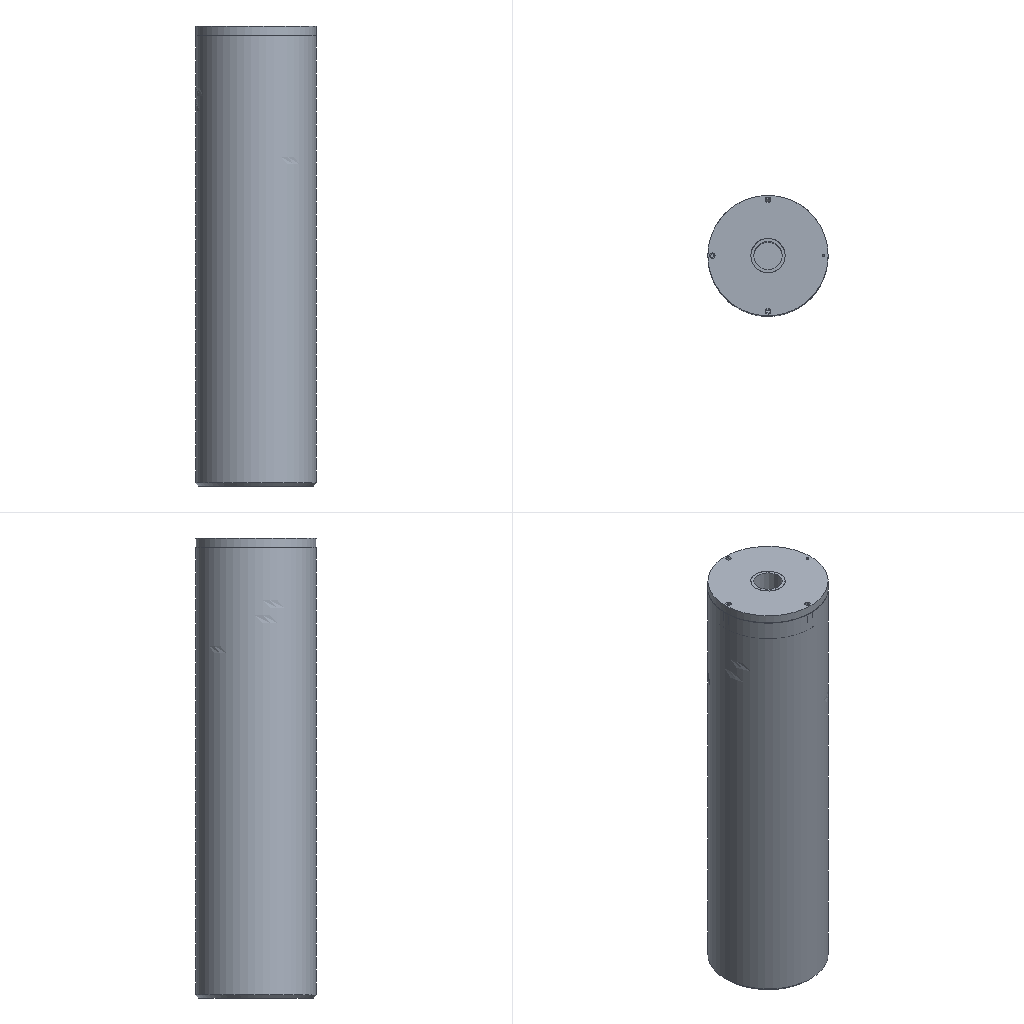Simulation study | abaqus
Set-up summary:
category,name,step,type,value,unit,region
solver,abaqus
solver,version,,,Abaqus/Explicit 2020
units,not stated in the deck,,not stated
analysis,deck,,transient,transient
load_step,Step-1,Step-1,transient,nlgeom=True
load_step,Step-2,Step-2,transient,nlgeom=True
contact,interactions,,,general=1 pairs=0 ties=1
load_step,requested,,,2
mesh,nodes,,,19414
mesh,elements,,,49290
element_type,C3D4,,solid,46469
element_type,C3D8R,,solid,2821
load,load commands in deck,,count,2
bc,support commands in deck,,count,1
material,C,,in results
material,C-COPY,,in results
check,setup vs results,,match,"per instance, exact: element labels, types and connectivity; labels of the nodes the elements use; coordinates of those nodes at SINGLE_PRECISION in 4 of 5 instance(s)"
Abaqus input file, long lists of numbers shortened:
*Heading
** Job name: Job-2 Model name: Model-1
** Generated by: Abaqus/CAE 2020
*Preprint, echo=NO, model=NO, history=NO, contact=NO
**
** PARTS
**
*Part, name=work-1
*Node
      1,         -32.,           0.,           2.
      2,         -34.,           0.,           4.
** (5795 more lines like these left out)
*Element, type=C3D4
    1, 5690, 5691,  279, 3044
    2, 5690, 5692,  207, 3074
** (17435 more lines like these left out)
*Nset, nset=Set-1, generate
    1,  5797,     1
*Elset, elset=Set-1, generate
     1,  17437,      1
** Section: c
*Solid Section, elset=Set-1, material=c
,
*End Part
**
*Part, name=work-2
*Node
      1,  -33.254,   13.79,          -2.
      2,  -35.102,   14.556,           0.
** (6591 more lines like these left out)
*Element, type=C3D4
    1,  864, 6155, 6156, 6205
    2,  800,  799,  848, 6188
** (19868 more lines like these left out)
*Nset, nset=Set-1, generate
    1,  6593,     1
*Elset, elset=Set-1, generate
     1,  19870,      1
*Nset, nset=Set-5, generate
    1,  6593,     1
*Elset, elset=Set-5, generate
     1,  19870,      1
** Section: Section-2
*Solid Section, elset=Set-5, material=c-Copy
,
*End Part
**
*Part, name=work-3
*Node
      1,          26.,           0.,         293.
      2,         -26.,           0.,         294.
** (1656 more lines like these left out)
*Element, type=C3D4
   1, 1075, 1076,  408, 1077
   2,  408, 1075, 1078, 1079
** (6524 more lines like these left out)
*Nset, nset=Set-1, generate
    1,  1658,     1
*Elset, elset=Set-1, generate
    1,  6526,     1
** Section: Section-2
*Solid Section, elset=Set-1, material=c-Copy
,
*End Part
**
*Part, name=work-8
*Node
      1,         -31.,           0.,           2.
      2,         -34.,           0.,           5.
** (672 more lines like these left out)
*Element, type=C3D4
   1, 419, 348, 420, 308
   2, 419, 348, 421, 420
** (2634 more lines like these left out)
*Nset, nset=Set-1, generate
   1,  674,    1
*Elset, elset=Set-1, generate
    1,  2636,     1
** Section: Section-2
*Solid Section, elset=Set-1, material=c-Copy
,
*End Part
**
*Part, name=work-9
*Node
      1,   8.927,   3.249,           2.
      2,         4.75,   8.227,           2.
** (4690 more lines like these left out)
*Element, type=C3D8R
   1,   53,   92,   65,   83,    2,   41,   14,   32
   2,   54,   77,  102,   93,    3,   26,   51,   42
** (2819 more lines like these left out)
*Nset, nset=Set-1, generate
    1,  4692,     1
*Elset, elset=Set-1, generate
    1,  2821,     1
** Section: c
*Solid Section, elset=Set-1, material=c
,
*End Part
**
**
** ASSEMBLY
**
*Assembly, name=Assembly
**
*Instance, name=work-1-1, part=work-1
*End Instance
**
*Instance, name=work-2-1, part=work-2
*End Instance
**
*Instance, name=work-3-1, part=work-3
*End Instance
**
*Instance, name=work-8-1, part=work-8
*End Instance
**
*Instance, name=work-9-1, part=work-9
*End Instance
**
*Node
      1,         300.,           0.,         150.
*Node
      2, 3.44435591e-12, 3.55883705e-14,         157.
*Nset, nset=Set-1, instance=work-2-1
   3, 103, 104, 105, 106, 107, 108, 109, 110, 111, 112, 113, 114, 115, 116, 117
 118, 119, 120, 121, 122, 123, 124, 125, 126, 127, 128, 129, 130, 131, 132, 133
** (14 more lines like these left out)
*Elset, elset=Set-1, instance=work-2-1
   853,  3663,  4359,  5785,  7353,  7354,  8199,  8345,  8349,  8365,  8392,  8404,  8871,  8984,  9069,  9093
  9136,  9151,  9156,  9163,  9173,  9174,  9223,  9832,  9878,  9880,  9910,  9911,  9920,  9929,  9951,  9965
** (27 more lines like these left out)
*Nset, nset=m_Set-2
 1,
*Nset, nset=m_Set-3
 2,
*Elset, elset=_m_Surf-3_S3, internal, instance=work-1-1
     3,     4,    18,    36,    40,    65,    81,    91,   133,   134,   142,   143,   145,   148,   150,   166
   178,   182,   186,   239,   258,   268,  7757,  7762,  7764,  7765,  7769,  7840,  7841,  7858,  7862,  7866
** (4 more lines like these left out)
*Elset, elset=_m_Surf-3_S3, internal, instance=work-2-1
    40,    47,    55,    64,    84,    88,   131,   138,   167,   180,   207,   457,   472,   498,   501,   513
   590,   606,   607,   652,  1246,  6379,  8322, 10268, 12947, 13296, 14264, 15517
*Elset, elset=_m_Surf-3_S2, internal, instance=work-1-1
   181,  7904,  8367,  8510,  9011,  9072,  9074, 11468, 11879, 16131, 16391, 17222
*Elset, elset=_m_Surf-3_S2, internal, instance=work-2-1
   158,   314,   376,   462,   532,   538,   565,  2683,  2783,  7103,  9781, 13212, 13462, 15843, 15854, 16126
 16978, 18548, 18936
*Elset, elset=_m_Surf-3_S4, internal, instance=work-1-1
   218,  7872,  7878,  7923,  8514,  8518,  8548,  8607,  8643,  8644,  8864,  8873,  8997,  9056,  9059,  9062
 11611, 16893, 17047, 17118
*Elset, elset=_m_Surf-3_S4, internal, instance=work-2-1
   443,   584,   637,   706,   729,   756,  7676,  9536,  9757,  9797, 10659, 13796, 14363, 14854, 16586, 18673
 19186,
*Elset, elset=_m_Surf-3_S1, internal, instance=work-1-1
  7315,  7848,  8503,  8655,  8791,  9047,  9057,  9060,  9071,  9092,  9098,  9137, 11612, 13123, 17011
*Elset, elset=_m_Surf-3_S1, internal, instance=work-2-1
    48,    73,    83,   187,   303,   406,   418,   435,   439,   441,   446,   447,   449,   465,   490,   492
   528,   555,   558,   561,   564,   567,   574,   619,   697,  2494,  2951,  3371,  6754, 11243, 12667, 13278
** (1 more lines like these left out)
*Elset, elset=_m_Surf-3_S1, internal, instance=work-9-1, generate
 2791,  2821,     1
*Surface, type=ELEMENT, name=m_Surf-3
_m_Surf-3_S3, S3
_m_Surf-3_S2, S2
_m_Surf-3_S4, S4
_m_Surf-3_S1, S1
*Elset, elset=_s_Surf-1_S3, internal, instance=work-2-1
     1,    25,    38,    51,    66,    71,    85,    86,   114,   119,   139,   158,   184,   185,   253,   254
   258,   259,   264,   267,   280,   282,   297,   301,   309,   317,   318,   325,   332,   339,   340,   343
** (57 more lines like these left out)
*Elset, elset=_s_Surf-1_S2, internal, instance=work-2-1
     9,    60,    63,    83,    91,    94,   102,   131,   133,   138,   175,   179,   180,   182,   200,   276
   295,   308,   346,   348,   354,   358,   368,   369,   370,   375,   379,   383,   399,   412,   431,   433
** (132 more lines like these left out)
*Elset, elset=_s_Surf-1_S4, internal, instance=work-2-1
    16,    20,    21,    59,    61,    64,    90,   187,   216,   222,   224,   298,   319,   361,   397,   420
   467,   470,   480,   482,   491,   492,   522,   528,   536,   539,   544,   549,   550,   578,   612,   615
** (96 more lines like these left out)
*Elset, elset=_s_Surf-1_S1, internal, instance=work-2-1
    23,    32,    46,    55,    88,   147,   152,   172,   197,   201,   218,   240,   256,   274,   288,   376
   415,   422,   437,   458,   462,   537,   540,   591,   605,   648,   651,   756,   770,   808,   816,   834
** (77 more lines like these left out)
*Surface, type=ELEMENT, name=s_Surf-1
_s_Surf-1_S3, S3
_s_Surf-1_S2, S2
_s_Surf-1_S4, S4
_s_Surf-1_S1, S1
*Elset, elset=_s_Surf-2_S3, internal, instance=work-9-1
    2,    7,   12,   18,   33,   38,   43,   49,   64,   69,   74,   80,   95,  100,  105,  111
  126,  131,  136,  142,  157,  162,  167,  173,  188,  193,  198,  204,  219,  224,  229,  235
** (21 more lines like these left out)
*Elset, elset=_s_Surf-2_S4, internal, instance=work-9-1
    4,    5,    6,   10,   11,   19,   24,   31,   35,   36,   37,   41,   42,   50,   55,   62
   66,   67,   68,   72,   73,   81,   86,   93,   97,   98,   99,  103,  104,  112,  117,  124
** (44 more lines like these left out)
*Elset, elset=_s_Surf-2_S6, internal, instance=work-9-1
    8,   15,   20,   27,   29,   39,   46,   51,   58,   60,   70,   77,   82,   89,   91,  101
  108,  113,  120,  122,  132,  139,  144,  151,  153,  163,  170,  175,  182,  184,  194,  201
** (27 more lines like these left out)
*Elset, elset=_s_Surf-2_S5, internal, instance=work-9-1, generate
   13,  2803,    31
*Surface, type=ELEMENT, name=s_Surf-2
_s_Surf-2_S3, S3
_s_Surf-2_S4, S4
_s_Surf-2_S6, S6
_s_Surf-2_S5, S5
*Elset, elset=_s_Surf-3_S4, internal, instance=work-3-1
    7,   49,  117,  377,  420,  640, 1016, 1105, 1422, 1485, 1505, 1644, 1699, 1707, 1726, 1799
 1819, 1825, 1852, 1877, 1918, 1952, 1956, 1962, 2062, 2069, 2085, 2154, 2170, 2174, 2247, 2258
** (3 more lines like these left out)
*Elset, elset=_s_Surf-3_S3, internal, instance=work-3-1
   19,   29,  205,  314,  431,  460,  598,  611,  642,  689,  713,  715,  814,  842,  873,  948
  960,  987, 1001, 1029, 1031, 1054, 1101, 1119, 1123, 1180, 1185, 1212, 1234, 1247, 1317, 1319
** (38 more lines like these left out)
*Elset, elset=_s_Surf-3_S2, internal, instance=work-3-1
  157,  267,  418, 1090, 1290, 1415, 1677, 1703, 1784, 1839, 1855, 1900, 1905, 1909, 1920, 1962
 1997, 2029, 2031, 2103, 2113, 2132, 2157, 2159, 2164, 2171, 2206, 2226, 2227, 2229, 2267, 2413
** (3 more lines like these left out)
*Elset, elset=_s_Surf-3_S1, internal, instance=work-3-1
    4,  839,  865, 1145, 1171, 1186, 1231, 1252, 1430, 1445, 1523, 1624, 1668, 1689, 1707, 1740
 1767, 1828, 1925, 1929, 1973, 1990, 2044, 2047, 2048, 2056, 2087, 2129, 2149, 2150, 2189, 2191
** (3 more lines like these left out)
*Surface, type=ELEMENT, name=s_Surf-3
_s_Surf-3_S4, S4
_s_Surf-3_S3, S3
_s_Surf-3_S2, S2
_s_Surf-3_S1, S1
*Elset, elset=_s_Surf-5_S4, internal, instance=work-1-1
   194,   277,   288,   291,   297,   298,   299,   306,   321,   326,   340,   343,   352,   361,   392,   394
   409,   420,   428,   448,   456,   459,   466,   474,   482,   494,   504,   513,   516,   518,   519,   524
** (96 more lines like these left out)
*Elset, elset=_s_Surf-5_S1, internal, instance=work-1-1
    68,   273,   278,   281,   283,   290,   295,   301,   317,   325,   332,   333,   342,   346,   351,   353
   354,   356,   360,   362,   363,   364,   373,   379,   384,   386,   389,   391,   398,   412,   423,   440
** (87 more lines like these left out)
*Elset, elset=_s_Surf-5_S2, internal, instance=work-1-1
   280,   303,   310,   324,   331,   337,   341,   348,   357,   366,   368,   371,   374,   385,   396,   401
   406,   410,   411,   415,   417,   429,   432,   476,   477,   480,   490,   491,   502,   536,   538,   552
** (132 more lines like these left out)
*Elset, elset=_s_Surf-5_S3, internal, instance=work-1-1
    73,   279,   372,   378,   380,   427,   433,   436,   441,   501,   507,   512,   542,   565,   592,   662
   669,   675,   681,   700,   703,   704,   710,   714,   772,   780,   805,   845,   862,   867,   893,   896
** (37 more lines like these left out)
*Surface, type=ELEMENT, name=s_Surf-5
_s_Surf-5_S4, S4
_s_Surf-5_S1, S1
_s_Surf-5_S2, S2
_s_Surf-5_S3, S3
** Constraint: Constraint-1
*Tie, name=Constraint-1, adjust=yes
s_Surf-3, m_Surf-3
*End Assembly
**
** MATERIALS
**
*Material, name=c
*Damage Initiation, criterion=SHEAR
 5e-05,0.,0.
*Damage Evolution, type=DISPLACEMENT
 1e-05,
*Density
 1.2e-09,
*Elastic
18000., 0.3
*Plastic
100.,0.
*Material, name=c-Copy
*Density
 1.2e-09,
*Elastic
18000., 0.3
*Plastic
100.,0.
**
** INTERACTION PROPERTIES
**
*Surface Interaction, name=IntProp-1
*Friction
 0.15,
*Surface Behavior, pressure-overclosure=HARD
*Incident Wave Interaction Property, name=IntProp-2, type=AIR BLAST
*CONWEP Charge Property
1e-05, 1000.
0.001, 1., 1e+06
*Incident Wave Interaction Property, name=IntProp-2-Copy, type=AIR BLAST
*CONWEP Charge Property
0.0001, 1000.
0.001, 1., 1e+06
** ----------------------------------------------------------------
**
** STEP: Step-1
**
*Step, name=Step-1, nlgeom=YES
*Dynamic, Explicit
, 0.001
*Bulk Viscosity
0.06, 1.2
**
** BOUNDARY CONDITIONS
**
** Name: BC-1 Type: 对称/反对称/完全固定
*Boundary
Set-1, ENCASTRE
**
** INTERACTIONS
**
** Interaction: Int-1
*Contact, op=NEW
*Contact Inclusions, ALL EXTERIOR
*Contact Property Assignment
 ,  , IntProp-1
** Interaction: Int-2
*Incident Wave Interaction, CONWEP, property=IntProp-2
s_Surf-1, m_Set-2,   , 0., 1.
**
** OUTPUT REQUESTS
**
*Restart, write, number interval=1, time marks=NO
**
** FIELD OUTPUT: F-Output-1
**
*Output, field
*Node Output
A, CF, RF, RM, RT, U, V
*Element Output, directions=YES
E, EVF, LE, MISES, MISESMAX, MISESONLY, NE, PE, PEEQ, PEEQMAX, PEEQT, PEEQVAVG, PEMAG, PEVAVG, PRESSONLY, S
SEQUT, SF, SSAVG, STATUS, SVAVG, YIELDPOT
*Contact Output
CDISP, CSTRESS
**
** HISTORY OUTPUT: H-Output-1
**
*Output, history, variable=PRESELECT
*End Step
** ----------------------------------------------------------------
**
** STEP: Step-2
**
*Step, name=Step-2, nlgeom=YES
*Dynamic, Explicit
, 0.001
*Bulk Viscosity
0.06, 1.2
**
** INTERACTIONS
**
** Interaction: Int-3
*Incident Wave Interaction, CONWEP, property=IntProp-2-Copy
s_Surf-5, m_Set-3,   , 0., 1.
**
** OUTPUT REQUESTS
**
*Restart, write, number interval=1, time marks=NO
**
** FIELD OUTPUT: F-Output-1
**
*Output, field
*Node Output
A, CF, RF, RM, RT, U, V
*Element Output, directions=YES
E, EVF, LE, MISES, MISESMAX, MISESONLY, NE, PE, PEEQ, PEEQMAX, PEEQT, PEEQVAVG, PEMAG, PEVAVG, PRESSONLY, S
SEQUT, SF, SSAVG, STATUS, SVAVG, YIELDPOT
*Contact Output
CDISP, CSTRESS
**
** HISTORY OUTPUT: H-Output-1
**
*Output, history, variable=PRESELECT
*End Step
Results summary:
result,step,Step-1,completed,increments=23386 time=0.001/0.001
result,step,Step-2,completed,increments=23380 time=0.001/0.001
result,analysis,,,transient
result,last_loadstep,,,2
result,analysis steps,,count,2
result,primary field,,,U
result,reaction total,,FX,6763.111,model units
result,reaction total,,FY,240.164,model units
result,reaction total,,FZ,602.102,model units